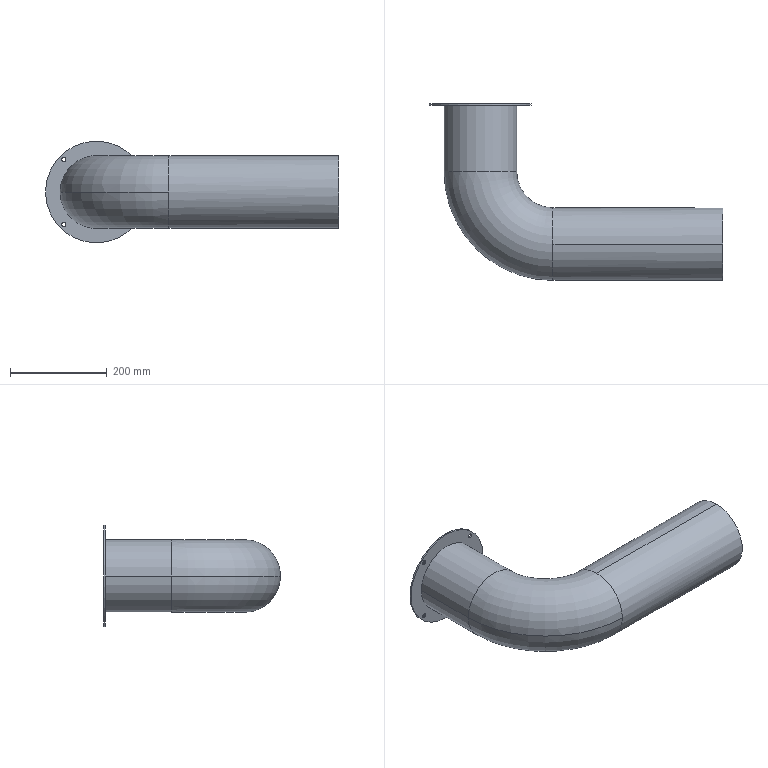Part | STEP file | Exhaust duct | 1 solid | 25 faces | box 605 x 365 x 210 mm | volume 724892 mm3 | cylinder 18 | torus 4 | plane 3 | commonest cylinder face diameters 9 x8 146 x4 150 x4 210 x2